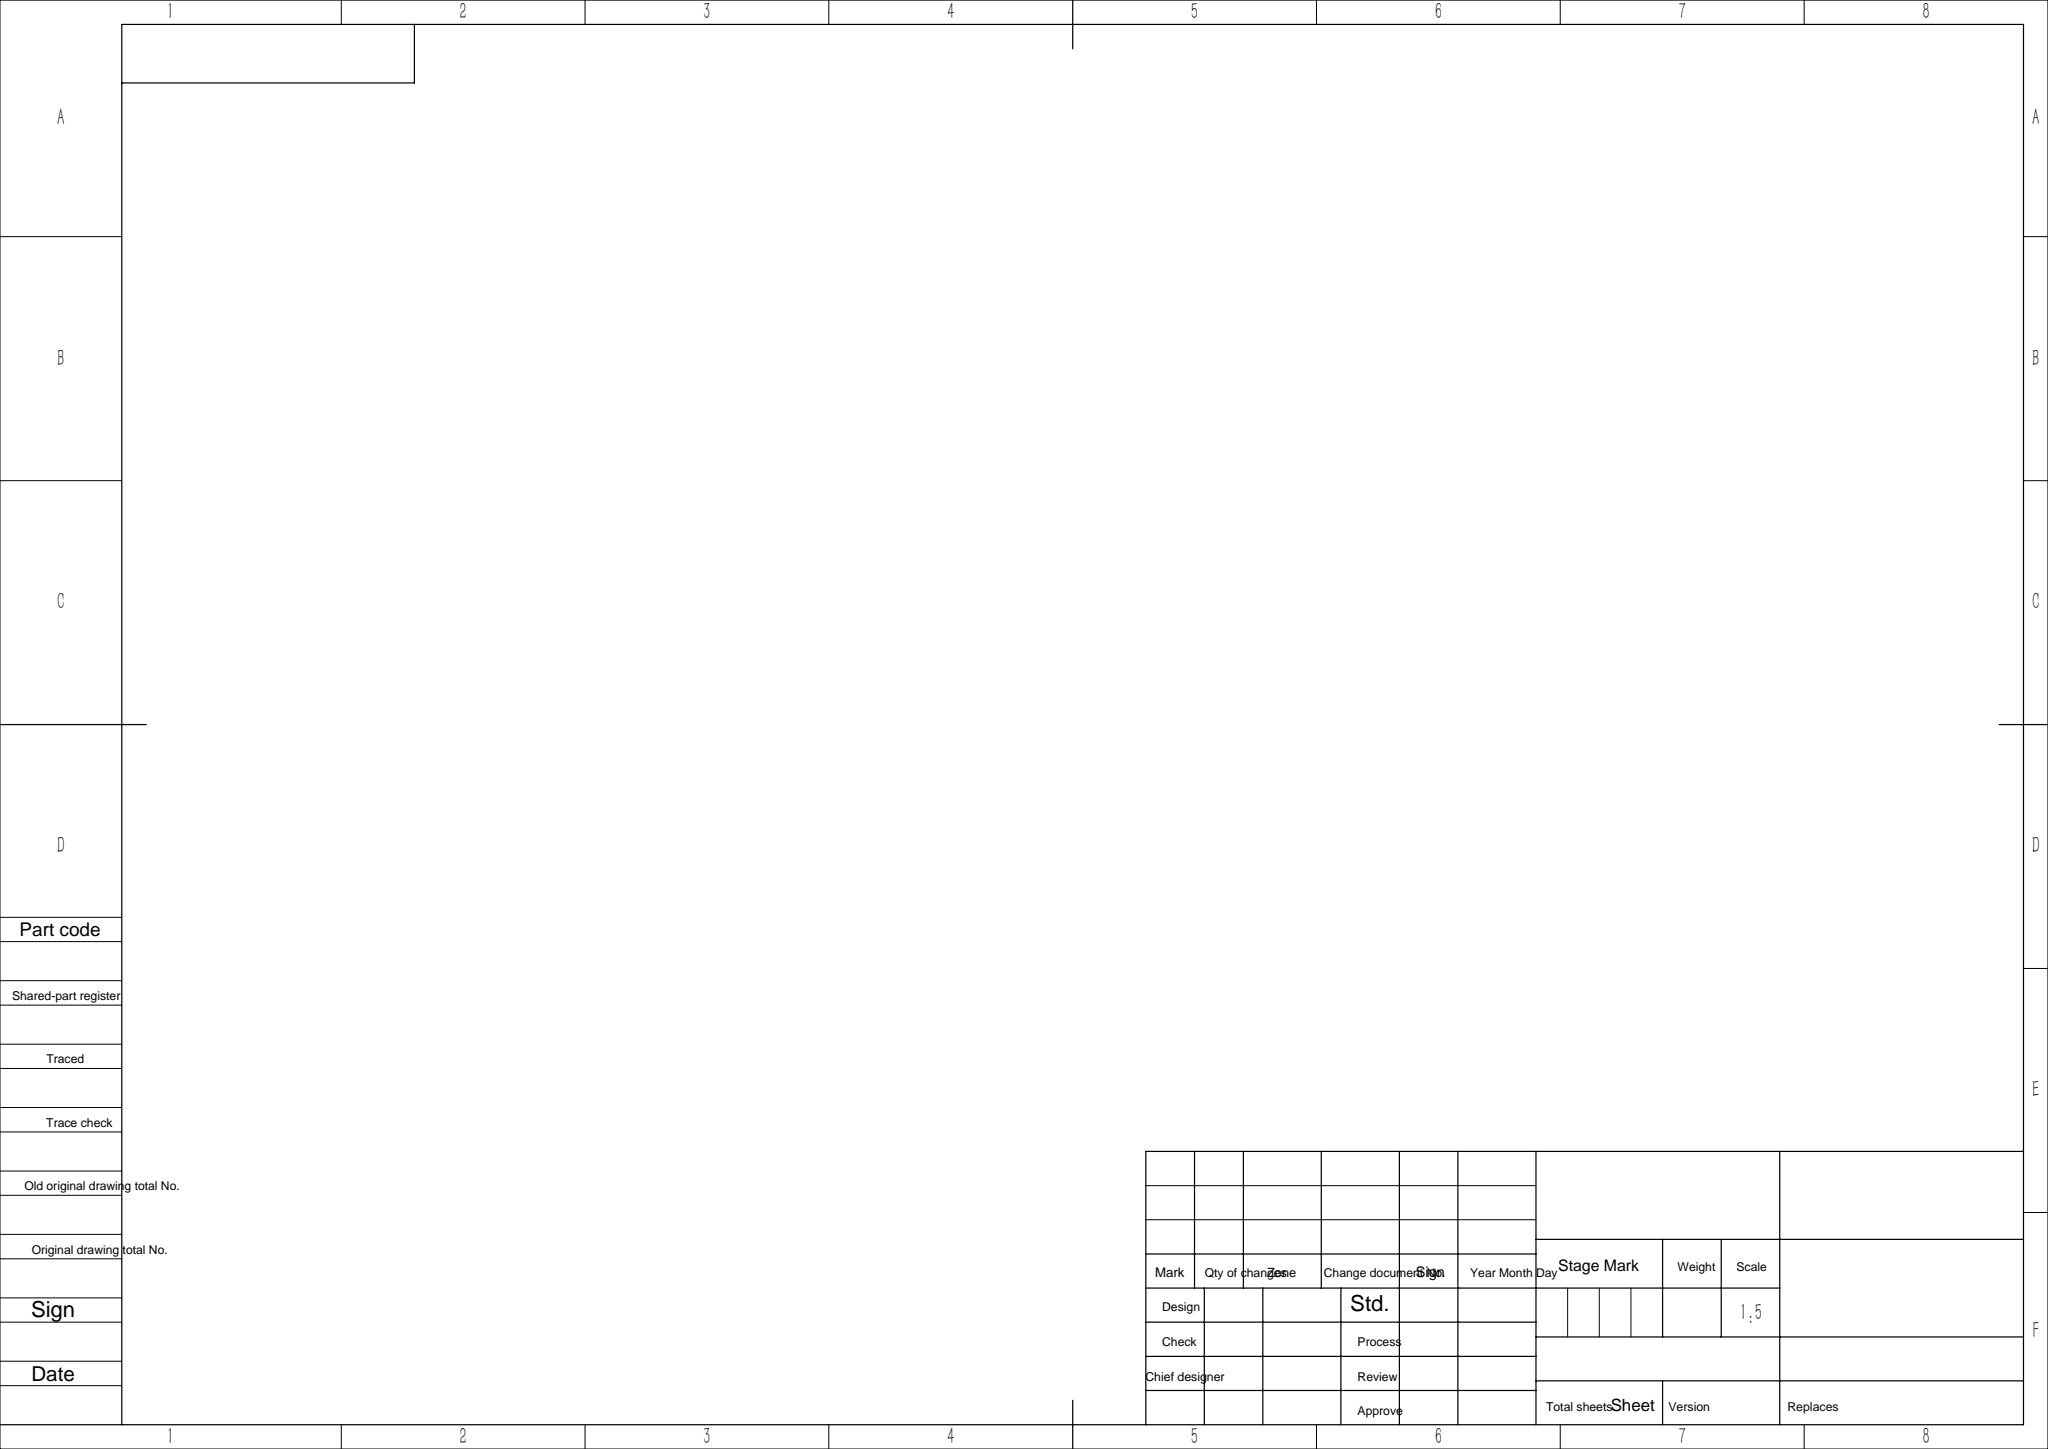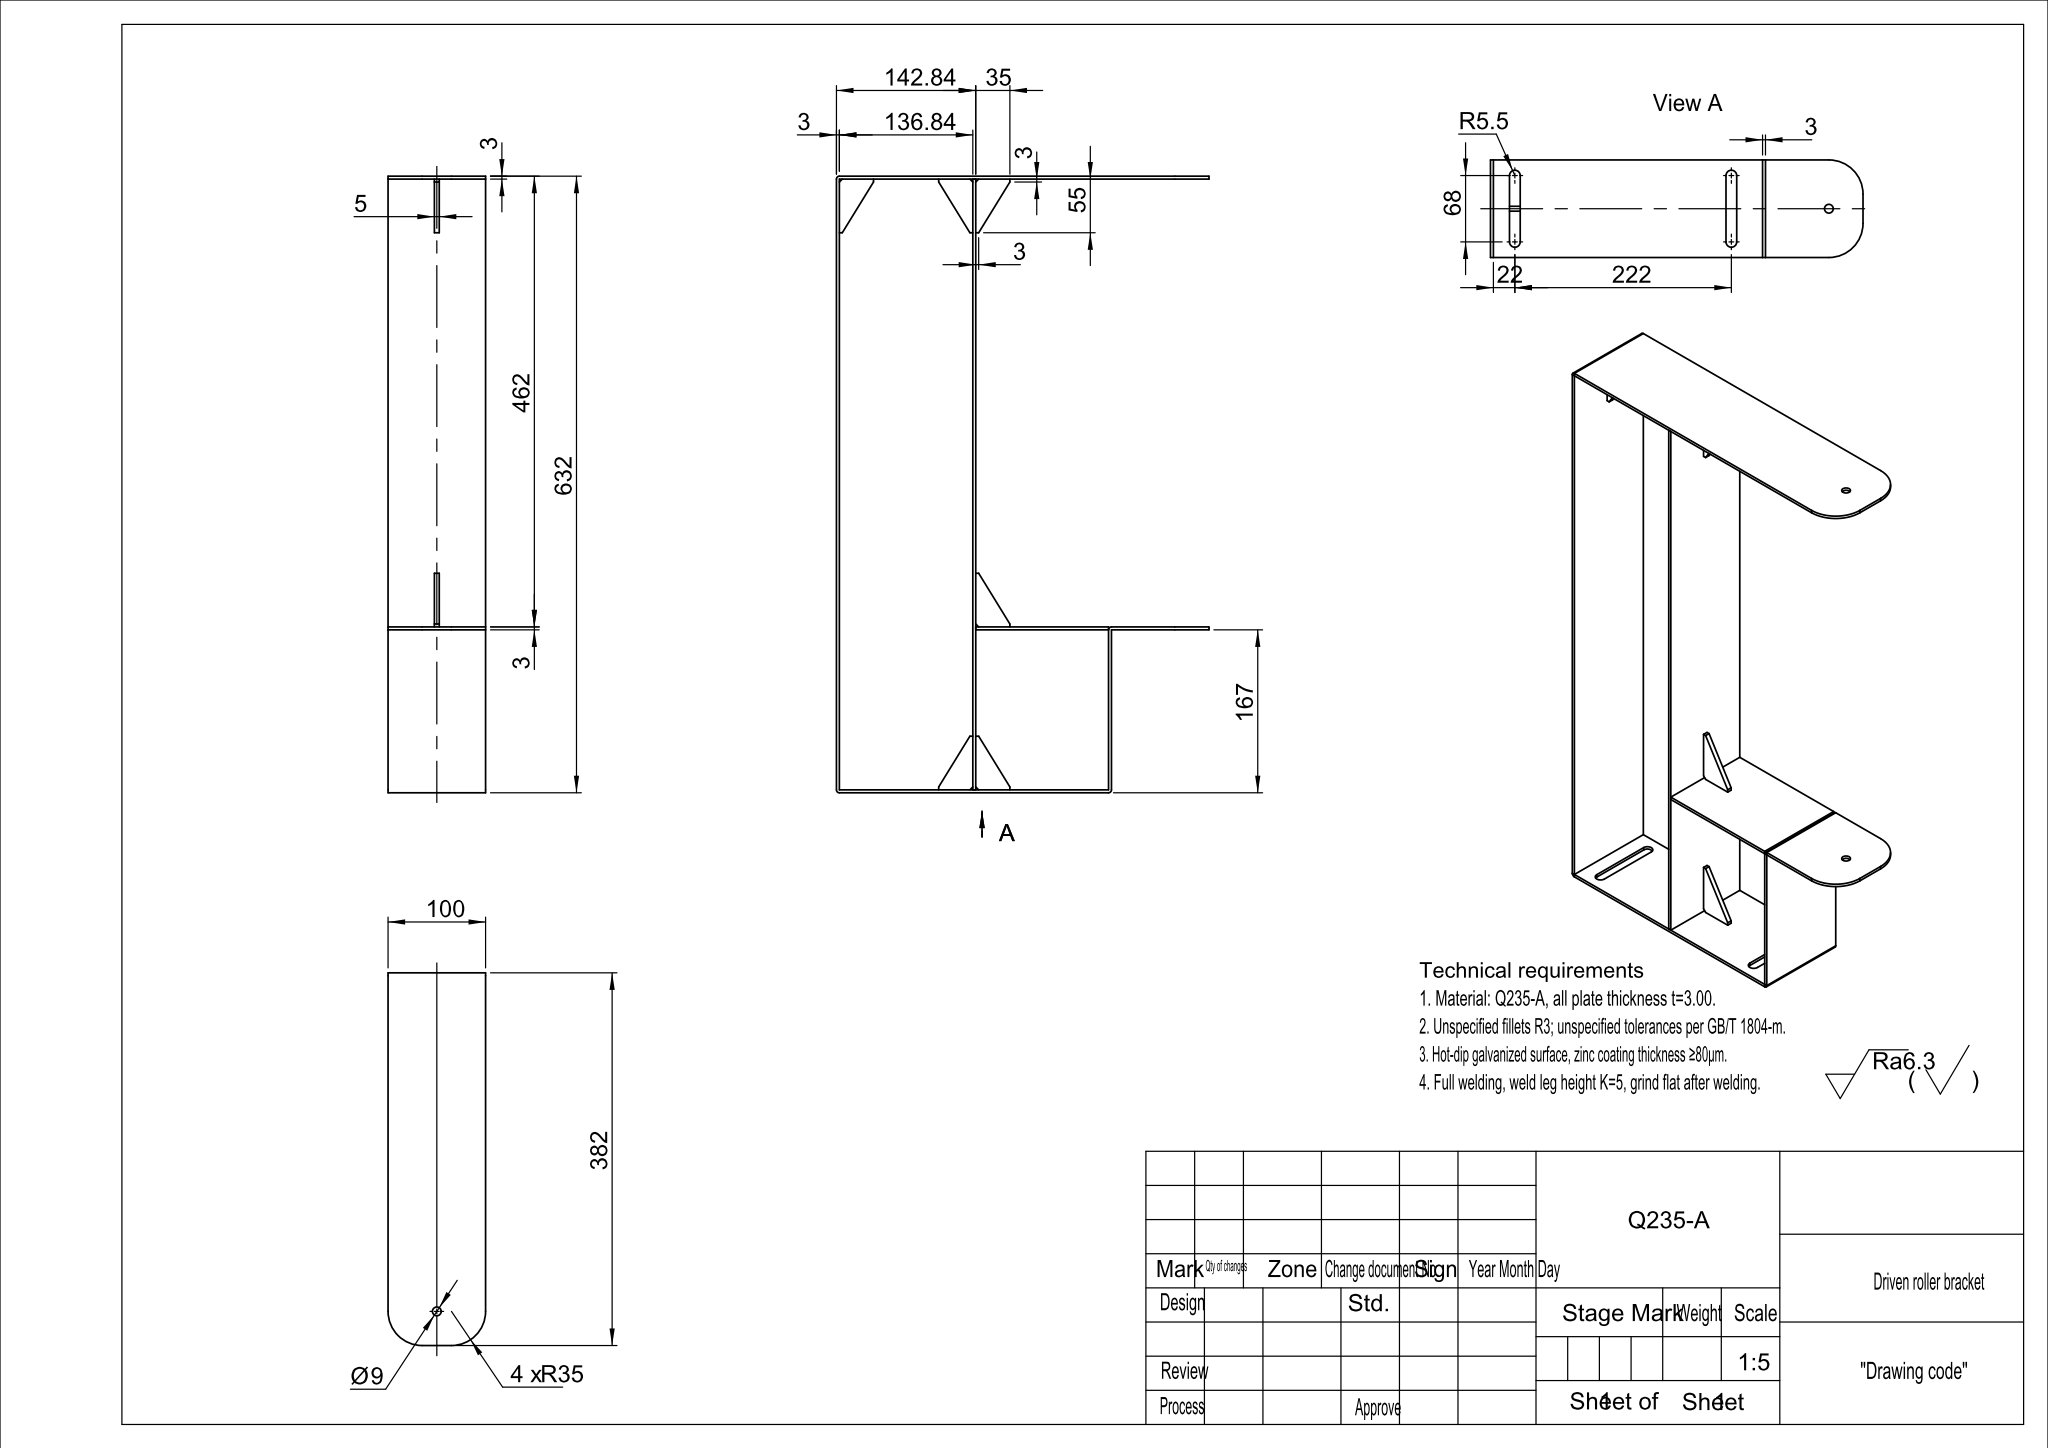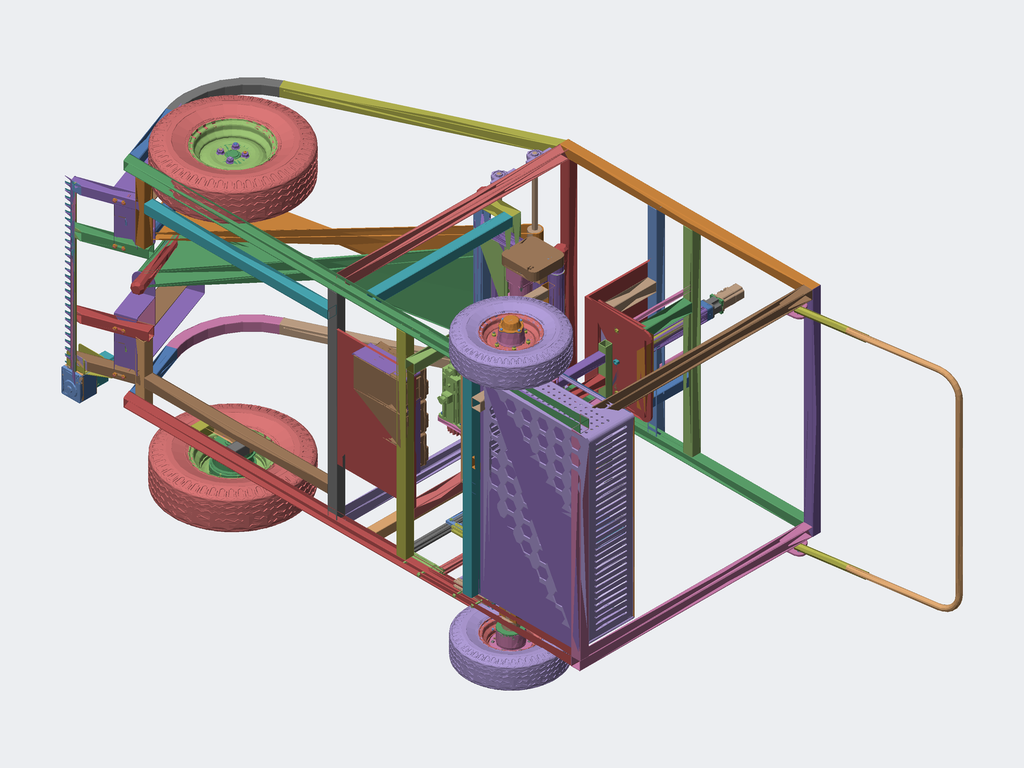Assembly | SolidWorks | 137 different items | 238 placed
Parts list (item | name | quantity | parent item | size | volume | features):
1 | (subassembly) | x1 | - | - | 4381513 mm3 | features CompositeCurve 5, ReferencePattern 5, MirrorCompFeat 1
2 | (subassembly) | x1 | in 1 | 56.95 x 46.85 x 36.783 mm | 5989 mm3 | -
3 | (subassembly) | x1 | - | 489 x 188.5 x 889 mm | 10301612 mm3 | -
4 | (subassembly) | x2 | in 5 | 193 x 193 x 273.493 mm | 3354612 mm3 | features ReferencePattern 14, LocalCirPattern 1
5 | (subassembly) | x2 | - | - | - | features ReferencePattern 3, LocalCirPattern 1
6 | (subassembly) | x2 | in 5 | - | - | -
7 | (subassembly) | x2 | - | - | - | -
8 | (subassembly) | x2 | in 7 | - | 1867736 mm3 | features ReferencePattern 26, LocalCirPattern 3, CompositeCurve 1
9 | (subassembly) | x1 | in 10 | 1039 x 6.076 x 81.5 mm | 84065 mm3 | -
10 | (subassembly) | x1 | - | 1053 x 226 x 197.5 mm | 1659148 mm3 | -
11 | (subassembly) | x1 | in 10 | 202.23 x 226 x 197.5 mm | 1360505 mm3 | -
12 | (subassembly) | x1 | in 13 | 30 x 30 x 35 mm | 19304 mm3 | -
13 | (subassembly) | x1 | - | 74.85 x 92 x 667.5 mm | 1531908 mm3 | features CompositeCurve 1
14 | (subassembly) | x1 | - | 477.948 x 507.594 x 700 mm | 2896175 mm3 | features ReferencePattern 17, LocalCirPattern 2, MirrorCompFeat 1
15 | (subassembly) | x1 | in 1 | 45 x 45 x 455.652 mm | 288434 mm3 | -
16 | (subassembly) | x3 | in 1 | 26 x 46 x 46 mm | 23618 mm3 | -
17 | - | x1 | in 10 | 915 x 11 x 28 mm | 111648 mm3 | features FlatPattern 3, SMBaseFlange 3, SheetMetal 3, HoleWzd 1, ICE 1, MoveFace 1
18 | - | x2 | in 7 | - | - | -
19 | - | x2 | - | 459 x 60 x 60 mm | 236387 mm3 | features BaseBody 1, RefAxis 1
20 | - | x2 | - | 1236 x 60 x 60 mm | 1636598 mm3 | features Chamfer 1, HoleWzd 1, Revolution 1
21 | - | x2 | - | 209.617 x 209.617 x 49 mm | 665029 mm3 | features ICE 5, CirPattern 2, Extrusion 1, Fillet 1, RefAxis 1
22 | - | x1 | - | 1396 x 1059 x 450 mm | 3582512 mm3 | features Blend 2, 3DProfileFeature 1, BossThin 1, ExtruThin 1
23 | - | x1 | - | 1406 x 865.848 x 450 mm | 9311838 mm3 | features Blend 2, BossThin 1, ExtruThin 1
24 | - | x1 | in 11 | 105 x 93 x 134 mm | 74755 mm3 | features Cut 2, FlatPattern 2, SMBaseFlange 2, SheetMetal 2, HoleWzd 1
25 | - | x1 | in 11 | 69 x 75 x 190 mm | 82445 mm3 | features ICE 3, SMBaseFlange 3, SM3dBend 2, Cut 1, Fillet 1, FlatPattern 1, SheetMetal 1
26 | - | x1 | in 11 | 69 x 124 x 116 mm | 64085 mm3 | features ICE 14, EdgeFlange 3, HoleWzd 2, FlatPattern 1, SM3dBend 1, SMBaseFlange 1, SheetMetal 1
27 | - | x1 | in 11 | 90 x 90 x 164.5 mm | 974524 mm3 | features BaseBody 1
28 | - | x1 | in 12 | 30 x 30 x 22.5 mm | 7880 mm3 | features BaseBody 1
29 | - | x1 | in 12 | 30 x 30 x 22.5 mm | 7120 mm3 | features BaseBody 1
30 | - | x1 | in 12 | 26.134 x 26.134 x 10 mm | 3952 mm3 | features BaseBody 1
31 | - | x1 | in 12 | 4 x 10 x 4 mm | 117.243 mm3 | features BaseBody 1
32 | - | x1 | in 12 | 10 x 4 x 4 mm | 117.243 mm3 | features BaseBody 1
33 | - | x1 | in 10 | 7 x 22 x 22 mm | 1715 mm3 | features Revolution 4, CirPattern 2, RefAxis 1, RevCut 1
34 | - | x1 | in 12 | 4 x 10 x 4 mm | 117.243 mm3 | features BaseBody 1
35 | - | x1 | in 13 | 60 x 72.85 x 148.5 mm | 399060 mm3 | features BaseBody 1
36 | - | x1 | in 13 | 64 x 92 x 13 mm | 47563 mm3 | features BaseBody 1
37 | - | x1 | in 13 | 28 x 29.8 x 29.8 mm | 11601 mm3 | features BaseBody 1
38 | - | x1 | in 13 | 64 x 64 x 52 mm | 89017 mm3 | features BaseBody 1
39 | - | x1 | in 13 | 429 x 30 x 30 mm | 140165 mm3 | features BaseBody 1, MoveFace 1
40 | - | x1 | in 13 | 63 x 63 x 398 mm | 629539 mm3 | features BaseBody 1
41 | - | x1 | in 13 | 64 x 64 x 34 mm | 81907 mm3 | features BaseBody 1
42 | - | x1 | in 13 | 64 x 64 x 49 mm | 81179 mm3 | features BaseBody 1
43 | - | x1 | in 13 | 33 x 26 x 3 mm | 2435 mm3 | features BaseBody 1
44 | - | x1 | in 10 | 35 x 31.385 x 31.157 mm | 18507 mm3 | features ICE 26, Fillet 5, CirPattern 4, Chamfer 2, Extrusion 2, Revolution 2
45 | - | x1 | in 13 | 64 x 64 x 14 mm | 28587 mm3 | features BaseBody 1
46 | - | x1 | in 13 | 15 x 17.321 x 9.5 mm | 1429 mm3 | features BaseBody 1
47 | - | x2 | - | 25 x 25 x 400 mm | 194835 mm3 | features Chamfer 1, Extrusion 1, HoleWzd 1
48 | - | x1 | - | 370 x 410 x 440 mm | 3370354 mm3 | features ICE 2, Extrusion 1, Fillet 1
49 | - | x2 | - | 62 x 62 x 59 mm | 52518 mm3 | features ICE 12, Fillet 2, Revolution 2, CirPattern 1, LPattern 1
50 | - | x1 | in 14 | 460 x 440 x 700 mm | 1262037 mm3 | features 3DProfileFeature 1, ICE 1, LPattern 1, WeldMemberFeat 1, WeldmentFeature 1
51 | - | x1 | in 14 | 460 x 340 x 660 mm | 1117739 mm3 | features 3DProfileFeature 1, CirPattern 1, HoleWzd 1, ICE 1, LPattern 1, MirrorPattern 1, MirrorSolid 1, SMBaseFlange 1, WeldMemberFeat 1, WeldmentFeature 1
52 | - | x1 | in 14 | 111 x 27.4 x 27.4 mm | 34833 mm3 | features ICE 4, HoleWzd 2, Chamfer 1, CirPattern 1, Helix 1, RefAxis 1, Revolution 1, SweepCut 1
53 | - | x1 | in 14 | 73.955 x 73.932 x 19.18 mm | 65019 mm3 | features CirPattern 2, Cut 1, Helix 1, HoleWzd 1, RefAxis 1, Revolution 1, SweepCut 1
54 | - | x2 | in 14 | 50 x 50 x 25.41 mm | 13372 mm3 | features ExtruThin 1, ICE 1, MirrorPattern 1
55 | - | x1 | in 9 | 74 x 6 x 78 mm | 14123 mm3 | features BaseBody 1, Cut 1, HoleWzd 1
56 | - | x1 | - | 16 x 16 x 730 mm | 145986 mm3 | features Extrusion 1, MirrorPattern 1, SweepThread 1
57 | - | x2 | in 1, 14 | 60 x 72 x 157 mm | 371769 mm3 | features ICE 23, Fillet 8, Chamfer 5, Extrusion 4, CirPattern 3, MirrorPattern 3, PLine 1, Revolution 1
58 | - | x6 | in 16 | 8 x 26 x 26 mm | 2677 mm3 | features Revolution 5, CirPattern 2, RefAxis 1, RevCut 1
59 | - | x1 | in 2 | 56.95 x 44.55 x 19.7 mm | 5255 mm3 | features BaseBody 8
60 | - | x1 | in 2 | 22.948 x 5.75 x 32.206 mm | 734.003 mm3 | features BaseBody 1
61 | - | x1 | in 15 | 32 x 32 x 312.5 mm | 42170 mm3 | features ICE 5, Revolution 3, RevCut 2, Chamfer 1, Helix 1, LPattern 1, MirrorPattern 1, SweepCut 1
62 | - | x1 | in 15 | 45 x 45 x 308 mm | 246238 mm3 | features ICE 10, Fillet 4, Revolution 4, MirrorPattern 3, Chamfer 2, CirPattern 2, Helix 1, RevCut 1, SweepCut 1
63 | - | x1 | in 1 | 37.938 x 37.788 x 30 mm | 21474 mm3 | features CirPattern 2, ICE 2, Extrusion 1, HoleWzd 1, RefAxis 1
64 | - | x1 | in 1 | 523.979 x 523.979 x 20 mm | 771365 mm3 | features ICE 2, CirPattern 1, Extrusion 1, HoleWzd 1, RefAxis 1
65 | - | x3 | in 16 | 26 x 46 x 46 mm | 18265 mm3 | features Chamfer 1, Fillet 1, Revolution 1
66 | - | x1 | in 9 | 984.736 x 2.5 x 55 mm | 69770 mm3 | features BaseBody 1, HoleWzd 1, ICE 1, MirrorSolid 1
67 | - | x1 | in 1 | 42 x 50 x 50 mm | 13320 mm3 | features Revolution 1
68 | - | x1 | in 1 | 12 x 50 x 50 mm | 5843 mm3 | features Revolution 1
69 | - | x1 | in 1 | 160 x 15 x 13 mm | 19723 mm3 | features Chamfer 1, ICE 1, MirrorPattern 1, Revolution 1, SweepThread 1
70 | - | x1 | in 1 | 80 x 80 x 40 mm | 150796 mm3 | features Extrusion 1
71 | - | x1 | in 1 | 525 x 737.5 x 40 mm | 2351947 mm3 | features ICE 4, WeldCornerFeat 2, WeldMemberFeat 1, WeldmentFeature 1
72 | - | x1 | in 1 | 80 x 92 x 44 mm | 20606 mm3 | features Gusset 2, EdgeFlange 1, Fillet 1, FlatPattern 1, ICE 1, SMBaseFlange 1, SheetMetal 1
73 | - | x1 | in 1 | 22 x 100 x 82 mm | 19719 mm3 | features Fillet 1, FlatPattern 1, ICE 1, SMBaseFlange 1, SheetMetal 1
74 | - | x1 | in 1 | 98 x 55 x 40 mm | 36160 mm3 | features EdgeFlange 3, CornerFeat 2, ICE 2, LPattern 2, FlatPattern 1, HoleWzd 1, MirrorSolid 1, MoveCopyBody 1, SMBaseFlange 1, SheetMetal 1, Stock 1
75 | - | x1 | in 1 | 200 x 90 x 10 mm | 96665 mm3 | features Chamfer 1, Extrusion 1, ICE 1
76 | - | x1 | in 1 | 12 x 12 x 300 mm | 32966 mm3 | features Chamfer 1, Extrusion 1, ICE 1, SweepThread 1
77 | - | x1 | in 10 | 915 x 2.5 x 55 mm | 63974 mm3 | features BaseBody 1, HoleWzd 1, ICE 1, MirrorSolid 1
78 | - | x3 | in 1 | 80 x 15 x 13 mm | 7147 mm3 | features Chamfer 1, ICE 1, MirrorPattern 1, Revolution 1, SweepThread 1
79 | - | x1 | in 1 | 42 x 42 x 30 mm | 10856 mm3 | features ICE 12, Fillet 2, Revolution 2, CirPattern 1, LPattern 1
80 | - | x1 | - | 130 x 178 x 321.686 mm | 3597344 mm3 | features ICE 34, Fillet 11, MirrorPattern 7, CirPattern 6, Revolution 4, Extrusion 3, PLine 3, Chamfer 2, Sweep 2
81 | - | x4 | - | 134 x 72.66 x 39.214 mm | 104404 mm3 | features Revolution 5, Cut 3, Boss 2, CirPattern 2, ICE 2, RevCut 2, Extrusion 1, RefAxis 1, SweepCut 1
82 | - | x2 | - | 382 x 632 x 100 mm | 719036 mm3 | features Gusset 6, FlatPattern 3, SMBaseFlange 3, SheetMetal 3, ICE 2, Fillet 1
83 | - | x1 | - | 109.134 x 109.134 x 50 mm | 234157 mm3 | features ICE 3, Chamfer 1, CirPattern 1, Extrusion 1, RefAxis 1
84 | - | x1 | - | 998.333 x 250 x 598.333 mm | 5087967 mm3 | features ICE 12, Fillet 6, Extrusion 1
85 | - | x1 | - | 1177 x 563.5 x 27 mm | 176772 mm3 | features Sweep 1
86 | - | x2 | - | 350 x 32 x 32 mm | 65429 mm3 | features ICE 1, Sweep 1
87 | - | x2 | - | 68.028 x 80 x 50 mm | 98491 mm3 | features Fillet 2, ICE 2, Extrusion 1, HoleWzd 1
88 | - | x1 | in 11 | 22 x 130 x 101 mm | 69870 mm3 | features ICE 10, Fillet 5, Chamfer 1, Extrusion 1, HoleWzd 1
89 | - | x1 | - | 2770 x 1437 x 1200 mm | 23055490 mm3 | features ICE 14, HoleWzd 6, Fillet 5, FlatPattern 4, CirPattern 3, Chamfer 2, Gusset 2, MirrorSolid 2, SMBaseFlange 2, SheetMetal 2, WeldCornerFeat 2, 3DProfileFeature 1, BossThin 1, LPattern 1, MirrorPattern 1, WeldMemberFeat 1, WeldmentFeature 1
90 | - | x3 | - | 270.928 x 169.188 x 160 mm | 6109502 mm3 | features ICE 22, Fillet 10, Chamfer 4, Blend 3, MirrorPattern 3, CirPattern 2, Extrusion 1
91 | - | x1 | in 3 | 95.773 x 92 x 218 mm | 1327877 mm3 | features RefAxis 54, 3DProfileFeature 18, ICE 8, Revolution 5, LPattern 2, Extrusion 1, RevCut 1
92 | - | x1 | in 3 | 485 x 86 x 861 mm | 7022086 mm3 | features ICE 76, Revolution 36, RefAxis 18, RevCut 18, LPattern 16, 3DProfileFeature 6, CombineBodies 1, MoveCopyBody 1, MoveFace 1, Scale 1
93 | - | x1 | in 3 | 195 x 186 x 53.5 mm | 223833 mm3 | features ICE 15, RefAxis 12, Revolution 8, 3DProfileFeature 4, LPattern 4, RevCut 3, Extrusion 1
94 | - | x1 | in 3 | 135.8 x 135.8 x 24.635 mm | 67609 mm3 | features RefAxis 3, Revolution 2, 3DProfileFeature 1, ICE 1
95 | - | x4 | in 3 | 10 x 10 x 91 mm | 2827 mm3 | features RefAxis 3, 3DProfileFeature 1, ICE 1, Revolution 1
96 | - | x1 | in 3 | 39.5 x 47 x 37 mm | 43916 mm3 | features RefAxis 3, ICE 2, 3DProfileFeature 1, Extrusion 1, RevCut 1, Revolution 1
97 | - | x2 | in 3 | 11.547 x 10 x 5 mm | 332.117 mm3 | features RefAxis 3, 3DProfileFeature 1, ICE 1, RevCut 1, Revolution 1
98 | - | x4 | in 3 | 12.5 x 12.5 x 3.1 mm | 284.047 mm3 | features RefAxis 3, 3DProfileFeature 1, RevCut 1, Revolution 1
99 | - | x1 | in 11 | 20.5 x 130 x 101 mm | 69425 mm3 | features ICE 9, Fillet 4, Chamfer 1, Extrusion 1, HoleWzd 1
100 | - | x1 | in 3 | 489 x 64 x 765 mm | 1603169 mm3 | features Extrusion 1
101 | - | x2 | in 4 | 190 x 190 x 186.81 mm | 3283817 mm3 | features CirPattern 2, HoleWzd 2, ICE 2, Chamfer 1, Revolution 1, SweepThread 1
102 | - | x2 | in 4 | 113.683 x 38.367 x 20 mm | 32123 mm3 | features ICE 1, Revolution 1, Sweep 1
103 | - | x2 | in 6 | 146.265 x 355.938 x 355.938 mm | 972609 mm3 | features ICE 1, Revolution 1
104 | - | x2 | in 5 | 70 x 10 x 40 mm | 23984 mm3 | features Extrusion 1, Fillet 1, HoleWzd 1
105 | - | x2 | in 6 | - | - | -
106 | - | x2 | in 8 | 44.037 x 50.85 x 26 mm | 23981 mm3 | features Cut 3, Chamfer 1, CirPattern 1, Extrusion 1
107 | - | x2 | in 8 | 56 x 4 x 56 mm | 6746 mm3 | features Revolution 1
108 | - | x2 | in 8 | 319 x 75 x 75 mm | 683914 mm3 | features Chamfer 4, Fillet 4, ICE 3, SweepThread 2, Cut 1, RefAxis 1, Revolution 1
109 | - | x2 | in 8 | 80 x 80 x 19.75 mm | 47853 mm3 | features Revolution 3, CirPattern 1, RefAxis 1
110 | - | x1 | in 10 | 30 x 55.5 x 47 mm | 14567 mm3 | features ICE 7, Chamfer 2, BaseBody 1
111 | - | x2 | in 8 | 110 x 110 x 23.75 mm | 99451 mm3 | features Revolution 3, CirPattern 1, RefAxis 1
112 | - | x2 | in 8 | 10 x 95 x 95 mm | 15410 mm3 | features Revolution 1
113 | - | x2 | in 8 | 120 x 120 x 1.5 mm | 4907 mm3 | features Extrusion 1
114 | - | x2 | in 8 | 18.4 x 10 x 11.547 mm | 670.595 mm3 | features Cut 1, Revolution 1
115 | - | x2 | in 8 | 21 x 120 x 120 mm | 65717 mm3 | features Revolution 1
116 | - | x2 | in 8 | 120 x 120 x 31.5 mm | 19269 mm3 | features Boss 1, Extrusion 1, Fillet 1, RefAxis 1, Shell 1
117 | - | x22 | in 8 | 12.785 x 15 x 47.6 mm | 3973 mm3 | features ICE 6, Chamfer 2, Fillet 2, Extrusion 1, Scale 1
118 | - | x22 | in 8 | 16.5 x 16.5 x 12.5 mm | 1193 mm3 | features Chamfer 2, Extrusion 1, Fillet 1, HoleWzd 1, ICE 1, RevCut 1, Revolution 1, Scale 1
119 | - | x2 | in 8 | 160 x 170 x 170 mm | 858037 mm3 | features Chamfer 3, Fillet 3, Draft 2, RevCut 2, Boss 1, CirPattern 1, Cut 1, HoleWzd 1, Revolution 1
120 | - | x2 | in 7 | 106.97 x 260.313 x 260.313 mm | 368325 mm3 | features ICE 2, Revolution 1, Scale 1
121 | - | x4 | - | 59.295 x 900 x 59.299 mm | 989144 mm3 | features Blend 1, Fillet 1, RefAxis 1
122 | cross recessed countersunk head screws gb2 | x1 | - | - | - | -
123 | cross recessed ctsk head screws type b gb | x1 | - | - | - | -
124 | hex flange bolts-heavy grade b gb | x1 | - | - | - | -
125 | hex lobular socket ctsk screws gb | x1 | - | - | - | -
126 | hex nuts, style 1-grades ab gb | x1 | - | - | - | -
127 | hexagon flange bolts--small series gb | x1 | - | - | - | -
128 | hexagon head bolts-full thread gb | x1 | - | - | - | -
129 | hexagon nuts with flange gb | x1 | - | - | - | -
130 | hexagon socket button head screws gb | x1 | - | - | - | -
131 | hexagon socket head cap screws gb | x1 | - | - | - | -
132 | plain washers-l series-grades ac gb | x1 | - | - | - | -
133 | plain washers-xl series-grade c gb | x1 | - | - | - | -
134 | round nuts gb | x1 | - | - | - | -
135 | split pins | x1 | - | - | - | -
136 | spring lock washers--normal type gb | x1 | - | - | - | -
137 | wing nuts gb | x1 | - | - | - | -
Mates (type | each side: item.copy, entity, surface, feature):
In the top assembly
Coincident | 89.1 plane | assembly plane | 3 times
Coincident | 66.1 face plane  Import 1 | assembly select_type:10
Parallel | 17.1 face plane Base-Flange 1 | assembly plane
DistanceDim | 24.1 face plane Base-Flange 1 | 89.1 face plane  Cold-Formed Hollow Square Tube gb/t6728-2002 50 X 50 X 1.5(1)
Coincident | 89.1 face plane  Cold-Formed Hollow Square Tube gb/t6728-2002 50 X 50 X 1.5(1) | 25.1 face plane Cut-Extrude 4
Coincident | 89.1 face plane  Cold-Formed Hollow Square Tube gb/t6728-2002 50 X 50 X 1.5(1) | 81.1 face plane Boss-Extrude 1
Width | 89.1 face plane  Cold-Formed Hollow Square Tube gb/t6728-2002 50 X 50 X 1.5(1) | 89.1 face plane  Cold-Formed Hollow Square Tube gb/t6728-2002 50 X 50 X 1.5(1) | 81.1 face plane Boss-Extrude 1 | 81.1 face plane Boss-Extrude 1
Concentric | 81.1 face cylinder Boss-Revolve 5 | 81.2 face cylinder Boss-Revolve 5
Coincident | 89.1 face plane  Cold-Formed Hollow Square Tube gb/t6728-2002 50 X 50 X 1.5(1) | 81.2 face plane Boss-Extrude 1
Width | 89.1 face plane  Cold-Formed Hollow Square Tube gb/t6728-2002 50 X 50 X 1.5(1) | 89.1 face plane  Cold-Formed Hollow Square Tube gb/t6728-2002 50 X 50 X 1.5(1) | 81.2 face plane Boss-Extrude 1 | 81.2 face plane Boss-Extrude 1
Coincident | 20.1 plane | assembly plane
Concentric | 81.1 face cylinder Boss-Revolve 5 | 20.1 face cylinder Revolve 1
DistanceDim | 19.1 face cylinder  Import 1 | 19.2 face cylinder  Import 1
DistanceDim | 81.2 face plane Boss-Extrude 1 | 89.1 face plane  Cold-Formed Hollow Square Tube gb/t6728-2002 50 X 50 X 1.5(1)
InPlace | 22.1 plane | assembly plane
InPlace | 23.1 plane | assembly plane
Concentric | 20.1 face cylinder Revolve 1 | 21.1 face cylinder Cut-Extrude 2
Concentric | 20.2 face cylinder Revolve 1 | 21.2 face cylinder Cut-Extrude 2
Coincident | 21.1 face plane Boss-Extrude 1 | 21.2 face plane Boss-Extrude 1
GearDim | 21.1 select_type:24 | 21.2 select_type:24
Coincident | 121.1 plane | assembly plane | 2 times
Coincident | 121.2 plane | assembly plane
Parallel | 121.2 axis | assembly select_type:10
Concentric | 19.1 face cylinder  Import 1 | 82.1 face cylinder Cut-Extrude 1
Coincident | 89.1 face plane  Cold-Formed Hollow Square Tube gb/t6728-2002 50 X 50 X 1.5(1) | 82.1 face plane Base-Flange 1
Coincident | 19.1 face plane  Import 1 | 82.1 face plane Base-Flange 1
Parallel | 89.1 face plane  Cold-Formed Hollow Square Tube gb/t6728-2002 50 X 50 X 1.5(1) | 82.1 face plane Base-Flange 1
Coincident | 14.1 plane | assembly plane
Coincident | 3.1 plane | assembly plane
DistanceDim | 92.1 face plane Boss-Extrude 6 | 89.1 face plane  Cold-Formed Hollow Square Tube gb/t6728-2002 50 X 50 X 1.5(1)
Coincident | 121.3 plane | assembly plane
Coincident | 121.4 plane | assembly plane
DistanceDim | 93.1 face plane Boss-Extrude 1 | 89.1 face plane  Cold-Formed Hollow Square Tube gb/t6728-2002 50 X 50 X 1.5(1)
Coincident | 89.1 face plane  Cold-Formed Hollow Square Tube gb/t6728-2002 50 X 50 X 1.5(1) | 71.1 face plane Aluminium Profile 30 X 30 X R2(1)
Width | 71.1 face plane Boss-Extrude 1 | 71.1 face plane Aluminium Profile 30 X 30 X R2(1) | 89.1 face plane  Cold-Formed Hollow Square Tube gb/t6728-2002 50 X 50 X 1.5(1) | 89.1 face plane  Cold-Formed Hollow Square Tube gb/t6728-2002 50 X 50 X 1.5(1)
Concentric | 89.1 face cylinder Cut-Extrude 4 | 71.1 face cylinder Cut-Extrude 3
Coincident | 89.1 face plane  Cold-Formed Hollow Square Tube gb/t6728-2002 50 X 50 X 1.5(1) | 50.1 face plane  Cold-Formed Hollow Square Tube gb/t6728-2002 40 X 40 X 1.5(1) | 2 times
Lock | 121.1 select_type:0 | 51.1 select_type:0
DistanceDim | 89.1 face plane  Cold-Formed Hollow Square Tube gb/t6728-2002 50 X 50 X 1.5(1) | 104.1 face plane Boss-Extrude 1
Width | 89.1 face plane  Cold-Formed Hollow Square Tube gb/t6728-2002 50 X 50 X 1.5(1) | 89.1 face plane  Cold-Formed Hollow Square Tube gb/t6728-2002 50 X 50 X 1.5(1) | 104.1 face plane Boss-Extrude 1 | 104.1 face plane Boss-Extrude 1
Concentric | 102.1 face cylinder Revolve 1 | 102.2 face cylinder Revolve 1
Width | 89.1 face plane  Cold-Formed Hollow Square Tube gb/t6728-2002 50 X 50 X 1.5(1) | 89.1 face plane  Cold-Formed Hollow Square Tube gb/t6728-2002 50 X 50 X 1.5(1) | 104.2 face plane Boss-Extrude 1 | 104.2 face plane Boss-Extrude 1
Parallel | 89.1 face plane  Cold-Formed Hollow Square Tube gb/t6728-2002 50 X 50 X 1.5(1) | 104.2 face plane Boss-Extrude 1
Concentric | 108.1 face cylinder Revolve 1 | 108.2 face cylinder Revolve 1
Coincident | 89.1 face plane  Cold-Formed Hollow Square Tube gb/t6728-2002 50 X 50 X 1.5(1) | 108.1 face plane Revolve 1
Coincident | 89.1 face plane  Cold-Formed Hollow Square Tube gb/t6728-2002 50 X 50 X 1.5(1) | 108.2 face plane Revolve 1
Coincident | 89.1 face plane  Cold-Formed Hollow Square Tube gb/t6728-2002 50 X 50 X 1.5(1) | 108.1 face plane Cut-Extrude 3
Coincident | 89.1 face plane Boss-Extrude 1 | 108.1 face plane Cut-Extrude 3
Coincident | 89.1 face plane Boss-Extrude 2 | 84.1 face plane Boss-Extrude 1
Coincident | 84.1 plane | assembly plane
Coincident | 89.1 face plane  Cold-Formed Hollow Square Tube gb/t6728-2002 50 X 50 X 1.5(1) | 84.1 face plane Cut-Extrude 2
Coincident | 48.1 plane | assembly plane
DistanceDim | 48.1 face plane Boss-Extrude 1 | 50.1 face plane  Cold-Formed Hollow Square Tube gb/t6728-2002 40 X 40 X 1.5(1)
Concentric | 48.1 face cylinder Cut-Extrude 1 | 37.1 face cylinder  Import 1
Coincident | 48.1 face plane Boss-Extrude 1 | 37.1 face plane  Import 1
Coincident | 89.1 face plane Boss-Extrude 4 | 36.1 face plane  Import 1
Parallel | 89.1 face plane Boss-Extrude 4 | 36.1 face plane  Import 1
Concentric | 89.1 face cylinder Cut-Extrude 5 | 49.1 face cylinder Revolve 1
Coincident | 89.1 face plane Boss-Extrude 4 | 49.1 face plane Revolve 1
Concentric | 89.1 face cylinder CirPattern 1 | 49.1 face cylinder Cut-Extrude 11
Concentric | 49.1 face cylinder Revolve 1 | 47.1 face cylinder Boss-Extrude 1
Coincident | 48.1 face plane Boss-Extrude 1 | 47.1 face plane Boss-Extrude 1
Coincident | 20.1 face plane Revolve 1 | 21.1 face plane Boss-Extrude 1
Concentric | 80.1 face cylinder Revolve 1 | 83.1 face cylinder Cut-Extrude 2
Coincident | 21.2 face plane Boss-Extrude 1 | 83.1 face plane Boss-Extrude 1
DistanceDim | 21.2 axis | 83.1 axis
Parallel | 89.1 face plane  Cold-Formed Hollow Square Tube gb/t6728-2002 50 X 50 X 1.5(1) | 80.1 face plane  Split Line 1
Coincident | 80.1 face plane Revolve 1 | 83.1 face plane Boss-Extrude 1
DistanceDim | 80.1 face cylinder Revolve 1 | 89.1 face plane  Cold-Formed Hollow Square Tube gb/t6728-2002 50 X 50 X 1.5(1)
GearDim | 21.2 select_type:24 | 83.1 select_type:24
Coincident | 56.1 plane | assembly plane
Concentric | 50.1 face cylinder Cut-Extrude 1 | 56.1 face cylinder Boss-Extrude 1
Coincident | 89.1 face plane Boss-Extrude 6 | 57.1 face plane Boss-Extrude 1
Coincident | 89.1 face plane Boss-Extrude 7 | 90.1 face plane Boss-Extrude 3
Width | 89.1 face plane Boss-Extrude 7 | 89.1 face plane Boss-Extrude 7 | 90.1 face plane Boss-Extrude 3 | 90.1 face plane Boss-Extrude 3
Coincident | 89.1 face plane Boss-Extrude 7 | 90.2 face plane Boss-Extrude 3
Coincident | 90.1 face plane Boss-Extrude 3 | 90.2 face plane Boss-Extrude 3 | 2 times
Coincident | 90.2 plane | assembly plane
Coincident | 89.1 face plane  Cold-Formed Hollow Square Tube gb/t6728-2002 50 X 50 X 1.5(1) | 87.1 face plane Boss-Extrude 1
Width | 89.1 face plane  Cold-Formed Hollow Square Tube gb/t6728-2002 50 X 50 X 1.5(1) | 89.1 face plane  Cold-Formed Hollow Square Tube gb/t6728-2002 50 X 50 X 1.5(1) | 87.1 face plane Boss-Extrude 1 | 87.1 face plane Boss-Extrude 1
Concentric | 89.1 face cylinder M10 Clearance Hole 1 | 87.1 face cylinder  Drill Hole Size (% per ) Hexalobular Socket Raised Countersunk Screw Type 1
Concentric | 87.1 face cylinder Cut-Extrude 2 | 86.1 face cylinder Cut-Extrude 1
Symmetric | 87.1 face plane Cut-Extrude 1 | 87.1 face plane Cut-Extrude 1 | 86.1 plane
Concentric | 86.1 face cylinder Sweep- Thin 1 | 85.1 face cylinder Sweep- Thin 1
Concentric | 86.2 face cylinder Sweep- Thin 1 | 85.1 face cylinder Sweep- Thin 1
In subassembly 7
Coincident | 120.1 select_type:24 | 7.1 plane | 2 times
Coincident | 120.1 plane | 7.1 plane
Coincident | 18.1 plane | 7.1 plane
Concentric | 120.1 face cylinder Revolve 1 | 18.1 face cylinder Revolve 1
Concentric | 120.1 face cylinder Revolve 1 | 119.1 face cylinder Revolve 1
Coincident | 120.1 face plane Revolve 1 | 119.1 face plane Revolve 1
Concentric | 120.1 face cylinder Cut-Extrude 2 | 119.1 face cylinder Cut-Extrude 2
Coincident | 120.1 face plane Revolve 1 | 118.1 face plane Boss-Extrude 1
In subassembly 8
Coincident | 108.3 plane | 8.1 plane | 3 times
Concentric | 108.3 face cylinder Revolve 1 | 111.1 face cylinder Revolve 1
Coincident | 108.3 face plane Revolve 1 | 111.1 face plane Revolve 1
Concentric | 108.3 face cylinder Revolve 1 | 109.1 face cylinder Revolve 1
Concentric | 108.3 face cylinder Revolve 1 | 119.2 face cone Revolve 1
Coincident | 111.1 face plane Revolve 3 | 119.2 face plane Revolve 1
Coincident | 109.1 face plane Revolve 3 | 119.2 face plane Revolve 1
Concentric | 115.1 face cylinder Revolve 2 | 112.1 face cylinder Revolve 1
Coincident | 115.1 face plane Revolve 2 | 112.1 face plane Revolve 1
Concentric | 108.3 face cylinder Revolve 1 | 115.1 face cylinder Revolve 2
Coincident | 115.1 face plane Revolve 2 | 119.2 face plane Revolve 1
Concentric | 108.3 face cylinder Revolve 1 | 107.1 face cylinder Base-Revolve
Coincident | 109.1 face plane Revolve 1 | 107.1 face plane Base-Revolve
Concentric | 108.3 face cylinder Revolve 1 | 106.1 face cylinder Base-Extrude
Coincident | 107.1 face plane Base-Revolve | 106.1 face plane Base-Extrude
Concentric | 108.3 face cylinder Revolve 1 | 113.1 face cylinder Boss-Extrude 1
Concentric | 113.1 face cylinder Boss-Extrude 1 | 119.2 face cylinder M8 Tapped Hole 2
Coincident | 113.1 face plane Boss-Extrude 1 | 119.2 face plane Revolve 1
Concentric | 116.1 face cylinder Boss-Extrude 1 | 119.2 face cylinder CirPattern 1
Concentric | 116.1 face cylinder Boss-Extrude 1 | 119.2 face cylinder M8 Tapped Hole 2
Coincident | 113.1 face plane Boss-Extrude 1 | 116.1 face plane Boss-Extrude 1
Concentric | 114.1 face cylinder Revolve 1 | 119.2 face cylinder Cut-Revolve 3
Coincident | 114.1 face plane Revolve 1 | 119.2 face plane Cut-Revolve 3
Concentric | 119.2 face cylinder Cut-Extrude 2 | 117.1 face cylinder Boss-Extrude 4
Coincident | 119.2 face plane Revolve 1 | 117.1 face plane Boss-Extrude 1
Concentric | 117.1 face cylinder Boss-Extrude 4 | 118.2 face cylinder M20x1.5 Tapped Hole 1
In subassembly 5
Concentric | 103.1 face cylinder Revolve 1 | 101.1 face cylinder Revolve 1
Concentric | 103.1 face cylinder Cut-Extrude 1 | 101.1 face cylinder Boss-Extrude 1
Coincident | 103.1 face plane Revolve 1 | 101.1 face plane Revolve 1
Coincident | 102.3 face plane Cut-Extrude 1 | 104.3 face plane Boss-Extrude 1
In subassembly 4
Coincident | 101.2 plane | 4.1 plane | 3 times
Concentric | 101.2 face cylinder Cut-Extrude 2 | 102.4 face cylinder Revolve 1
DistanceDim | 102.4 face plane Revolve 1 | 101.2 face plane Revolve 1
In subassembly 6
Coincident | 103.2 select_type:24 | 6.1 plane | 2 times
Coincident | 103.2 plane | 6.1 plane
Coincident | 105.1 plane | 6.1 plane
Concentric | 103.2 face cylinder Revolve 1 | 105.1 face cylinder Revolve 1
In subassembly 3
DistanceDim | 95.1 plane | 91.1 plane
Coincident | 91.1 axis | 95.1 axis | 3 times
PlanarAngleDim | 95.1 plane | 91.1 plane
DistanceDim | 95.2 plane | 91.1 plane
Coincident | 91.1 axis | 95.2 axis | 3 times
PlanarAngleDim | 95.2 plane | 91.1 plane
DistanceDim | 95.3 plane | 91.1 plane
Coincident | 91.1 axis | 95.3 axis | 3 times
PlanarAngleDim | 95.3 plane | 91.1 plane
DistanceDim | 95.4 plane | 91.1 plane
Coincident | 91.1 axis | 95.4 axis | 3 times
PlanarAngleDim | 95.4 plane | 91.1 plane
DistanceDim | 98.1 plane | 91.1 plane
Coincident | 91.1 axis | 98.1 axis | 3 times
PlanarAngleDim | 98.1 plane | 91.1 plane
DistanceDim | 98.2 plane | 91.1 plane
Coincident | 91.1 axis | 98.2 axis | 3 times
PlanarAngleDim | 98.2 plane | 91.1 plane
DistanceDim | 98.3 plane | 91.1 plane
Coincident | 91.1 axis | 98.3 axis | 3 times
PlanarAngleDim | 98.3 plane | 91.1 plane
DistanceDim | 98.4 plane | 91.1 plane
Coincident | 91.1 axis | 98.4 axis | 3 times
PlanarAngleDim | 98.4 plane | 91.1 plane
DistanceDim | 97.1 plane | 91.1 plane
Coincident | 91.1 axis | 97.1 axis | 3 times
PlanarAngleDim | 97.1 plane | 91.1 plane
DistanceDim | 97.2 plane | 91.1 plane
Coincident | 91.1 axis | 97.2 axis | 3 times
PlanarAngleDim | 97.2 plane | 91.1 plane
Concentric | 92.2 face cylinder Revolve 1 | 94.1 face cylinder Revolve 2
Coincident | 92.2 face plane Revolve 1 | 94.1 face plane Revolve 2
Concentric | 91.1 face cylinder Revolve 1 | 94.1 face cylinder Revolve 1
Concentric | 93.2 face cylinder Cut-Revolve 2 | 95.3 face cylinder Revolve 1
Parallel | 92.2 face plane Boss-Extrude 2 | 93.2 face plane Boss-Extrude 1
Coincident | 92.2 face plane Boss-Extrude 2 | 93.2 face plane Boss-Extrude 1 | 2 times
Coincident | 93.2 face plane Boss-Extrude 2 | 91.1 face plane Boss-Extrude 1
Parallel | 93.2 face plane Boss-Extrude 1 | 91.1 face plane Boss-Extrude 1 | 2 times
InPlace | 100.1 plane | 3.2 plane
Concentric | 93.2 face cylinder Cut-Revolve 3 | 96.1 face cylinder Revolve 1
Coincident | 93.2 face plane Boss-Extrude 2 | 96.1 face plane Boss-Extrude 1
Parallel | 93.2 face plane Boss-Extrude 1 | 96.1 face plane Boss-Extrude 1
In subassembly 1
Coincident | 71.2 plane | 1.1 plane | 3 times
Concentric | 71.2 select_type:24 | 64.1 face cylinder Cut-Extrude 2
DistanceDim | 64.1 axis | 63.1 axis
Coincident | 64.1 face plane Boss-Extrude 1 | 63.1 face plane Boss-Extrude 1
Coincident | 64.1 plane | 16.1 plane
Tangent | 64.1 face cylinder Cut-Extrude 2 | 65.1 face cylinder Revolve 1
Slot | 58.1 face cylinder Revolve 1 | 71.2 face plane Cut-Extrude 1
Concentric | 58.1 face cylinder Revolve 1 | 78.1 face cylinder Revolve 1
Coincident | 71.2 face plane Boss-Extrude 1 | 78.1 face plane Revolve 1
Coincident | 58.2 face plane Revolve 1 | 78.1 face plane Revolve 1
Concentric | 58.3 face cylinder Revolve 1 | 78.2 face cylinder Revolve 1
Coincident | 58.4 face plane Revolve 1 | 78.2 face plane Revolve 1
Coincident | 71.2 face plane Boss-Extrude 1 | 78.2 face plane Revolve 1
Slot | 78.2 face cylinder Revolve 1 | 71.2 face plane Cut-Extrude 1
Tangent | 64.1 face cylinder Cut-Extrude 2 | 65.2 face cylinder Revolve 1
Concentric | 64.1 face cylinder M10 Tapped Hole 1 | 69.1 face cylinder Revolve 1
Coincident | 64.1 face plane Boss-Extrude 1 | 69.1 face plane Revolve 1
Concentric | 69.1 face cylinder Revolve 1 | 67.1 face cylinder Revolve 1
Coincident | 69.1 face plane Revolve 1 | 67.1 face plane Revolve 1
Concentric | 67.1 face cylinder Revolve 1 | 68.1 face cylinder Revolve 1
Coincident | 67.1 face plane Revolve 1 | 68.1 face plane Revolve 1
Concentric | 67.1 face cylinder Revolve 1 | 70.1 face cylinder Boss-Extrude 1
Coincident | 67.1 face plane Revolve 1 | 70.1 face plane Boss-Extrude 1
Concentric | 62.1 face cylinder Cut-Extrude 10 | 75.1 edge
Concentric | 79.1 face cylinder Revolve 1 | 75.1 face cylinder Boss-Extrude 1
Concentric | 79.1 face cylinder Cut-Extrude 11 | 75.1 face cylinder Boss-Extrude 1
Coincident | 79.1 face plane Revolve 1 | 75.1 face plane Boss-Extrude 1
Coincident | 62.1 face plane Boss-Extrude 1 | 75.1 face plane Boss-Extrude 1
Coincident | 71.2 face plane Aluminium Profile 30 X 30 X R2(1) | 75.1 face plane Boss-Extrude 1
Concentric | 79.1 face cylinder Cut-Extrude 1 | 76.1 face cylinder Boss-Extrude 1
Concentric | 61.1 face cylinder Revolve 1 | 73.1 face cylinder Cut-Extrude 1
Concentric | 76.1 face cylinder Boss-Extrude 1 | 73.1 face cylinder Cut-Extrude 1
Coincident | 61.1 face plane Boss-Extrude 4 | 73.1 face plane Base-Flange 1
DistanceDim | 76.1 face plane Boss-Extrude 1 | 73.1 face plane Base-Flange 1
Concentric | 63.1 select_type:24 | 57.2 face cylinder Revolve 1
Parallel | 71.2 face plane Aluminium Profile 30 X 30 X R2(1) | 57.2 face plane  Split Line 1
Coincident | 63.1 axis | 1.1 plane
Concentric | 57.2 face cylinder Boss-Extrude 4 | 72.1 face cylinder Base-Flange 1
Concentric | 57.2 face cylinder CirPattern 3 | 72.1 face cylinder Base-Flange 1
Coincident | 57.2 face plane Boss-Extrude 1 | 72.1 face plane Base-Flange 1
GearDim | 64.1 select_type:24 | 63.1 select_type:24
Concentric | 62.1 face cylinder Cut-Extrude 10 | 74.1 face cylinder Base-Flange 1
Concentric | 75.1 face cylinder Cut-Extrude 1 | 74.1 face cylinder LPattern 2
Coincident | 75.1 face plane Boss-Extrude 1 | 74.1 face plane Base-Flange 1
Concentric | 59.1 face cylinder  Import 5 | 74.1 face cylinder M4 Tapped Hole 1 | 2 times
Coincident | 59.1 face plane  Import 5 | 74.1 face plane Boss-Extrude 1
DistanceDim | 75.1 face plane Boss-Extrude 1 | 71.2 face plane Aluminium Profile 30 X 30 X R2(1) | 2 times
Coincident | 71.2 face plane Aluminium Profile 30 X 30 X R2(1) | 72.1 face plane Edge-Flange 1
Parallel | 62.1 face plane Boss-Extrude 1 | 75.1 face plane Boss-Extrude 1
In subassembly 16
Coincident | 65.3 plane | 16.2 plane | 3 times
Coincident | 65.3 face plane Revolve 1 | 58.5 face plane Revolve 1
Coincident | 65.3 face plane Revolve 1 | 58.6 face plane Revolve 1
Concentric | 65.3 face cylinder Revolve 1 | 58.6 face cylinder Revolve 1
Concentric | 65.3 face cylinder Revolve 1 | 58.5 face cylinder Revolve 1
In subassembly 2
Coincident | 59.2 plane | 2.1 plane | 3 times
Concentric | 59.2 face cylinder  Import 5 | 60.1 face cylinder  Import 8
DistanceDim | 59.2 face plane  Import 5 | 60.1 face plane  Import 8
In subassembly 15
Concentric | 62.2 face cylinder Revolve 2 | 61.2 face cylinder Revolve 1
In subassembly 14
Coincident | 50.2 plane | 14.2 plane | 3 times
Coincident | 51.2 plane | 14.2 plane
Concentric | 50.2 face cylinder Cut-Extrude 1 | 51.2 face cylinder Cut-Extrude 1
LimitPlanarAngleDim | 50.2 face plane  Cold-Formed Hollow Square Tube gb/t6728-2002 40 X 40 X 1.5(1) | 51.2 face plane LPattern 1
Concentric | 51.2 face cylinder Cut-Extrude 1 | 53.1 face cylinder Revolve 1
Coincident | 53.1 plane | 14.2 plane
Coincident | 52.1 axis | 14.2 plane
DistanceDim | 52.1 axis | 53.1 axis
GearDim | 52.1 face cylinder Revolve 1 | 53.1 face cone Revolve 1
Concentric | 51.2 face cylinder Cut-Extrude 1 | 54.1 face cylinder Extrude- Thin-Wall 1
Coincident | 51.2 face plane LPattern 1 | 54.1 face plane Extrude- Thin-Wall 1
Concentric | 51.2 face cylinder M5 Tapped Hole 1 | 54.1 face cylinder Boss-Extrude 1
Concentric | 53.1 face cylinder M5 Tapped Hole 1 | 54.1 face cylinder Mirror 1
Concentric | 52.1 face cylinder Boss-Extrude 1 | 57.2 face cylinder Revolve 1
Parallel | 57.2 face plane  Split Line 1 | 14.2 plane
In subassembly 13
LimitDistanceDim | 37.2 face plane  Import 1 | 38.1 face plane  Import 1
Concentric | 38.1 face cylinder  Import 1 | 39.1 face cylinder  Import 1
Concentric | 39.1 face cylinder  Import 1 | 37.2 face cylinder  Import 1
Coincident | 39.1 face plane  Import 1 | 37.2 edge
In subassembly 10
Width | 88.1 face plane Boss-Extrude 1 | 88.1 face plane Boss-Extrude 1 | 55.1 face plane  Import 1 | 55.1 face plane  Import 1
Coincident | 17.2 face plane Base-Flange 1 | 77.1 face plane  Import 1
Coincident | 66.2 face plane  Import 1 | 77.1 face plane  Import 1
Width | 77.1 face plane  Import 1 | 66.2 face plane  Import 1 | 88.1 face plane Cut-Extrude 4 | 99.1 face plane Cut-Extrude 4
Width | 66.2 face plane  Import 1 | 66.2 face plane  Import 1 | 99.1 face plane Cut-Extrude 4 | 99.1 face plane Cut-Extrude 4
Coincident | 17.2 face plane Base-Flange 2 | 77.1 face plane  Import 1
Concentric | 99.1 face cylinder Cut-Extrude 6 | 110.1 face cylinder Boss-Extrude 7
Tangent | 55.1 face plane  Import 1 | 110.1 face cylinder  Import 5
Concentric | 27.1 face cylinder  Import 1 | 110.1 face cylinder Boss-Extrude 6
Concentric | 99.1 face cylinder Cut-Extrude 6 | 33.1 face cylinder Revolve 1
Coincident | 99.1 face plane Cut-Extrude 6 | 33.1 face plane Revolve 1
Coincident | 110.1 face plane Boss-Extrude 5 | 33.1 face plane Revolve 1
Concentric | 110.1 face cylinder Boss-Extrude 6 | 44.1 face cylinder Cut-Extrude 2
Parallel | 99.1 face plane Boss-Extrude 1 | 55.1 face plane  Import 1
Coincident | 17.2 plane | 10.1 plane | 3 times
DistanceDim | 44.1 face plane Revolve 1 | 27.1 face plane  Import 1
Coincident | 88.1 face plane Boss-Extrude 1 | 17.2 face plane Base-Flange 1
Coincident | 17.2 face plane Base-Flange 1 | 77.1 face plane Cut-Extrude 1
Coincident | 66.2 face plane  Import 1 | 17.2 face plane Base-Flange 2
In subassembly 11
Coincident | 26.1 face plane Edge-Flange 3 | 11.1 plane
Coincident | 26.1 face plane Edge-Flange 2 | 11.1 plane
Coincident | 26.1 plane | 11.1 plane
Coincident | 26.1 face plane Edge-Flange 1 | 25.2 face plane  Sketched Bend 2
Coincident | 26.1 face plane Edge-Flange 2 | 25.2 face plane Base-Flange 1 | 2 times
Slot | 26.1 face plane Cut-Extrude 10 | 27.2 face cylinder  Import 1
Slot | 27.2 face cylinder  Import 1 | 26.1 face plane Cut-Extrude 7
Coincident | 26.1 face plane Edge-Flange 1 | 27.2 face plane  Import 1
Concentric | 26.1 face cylinder Ø7.0 (7) DiameterHole 1 | 88.2 face cylinder Ø7.0 (7) DiameterHole 1 | 2 times
Coincident | 26.1 face plane Base-Flange 1 | 88.2 face plane Boss-Extrude 1
Concentric | 88.2 face cylinder Ø7.0 (7) DiameterHole 1 | 99.2 face cylinder M6 Tapped Hole 1 | 2 times
Coincident | 88.2 face plane Boss-Extrude 1 | 99.2 face plane Boss-Extrude 1
Width | 99.2 face plane Boss-Extrude 1 | 99.2 face plane Boss-Extrude 1 | 24.2 face plane Base-Flange 1 | 24.2 face plane Base-Flange 1
Coincident | 99.2 face plane Boss-Extrude 1 | 24.2 face plane Base-Flange 1 | 2 times
In subassembly 9
Coincident | 55.2 face plane Cut-Extrude 1 | 66.3 face plane  Import 1 | 3 times
Coincident | 66.3 plane | 9.1 plane | 3 times